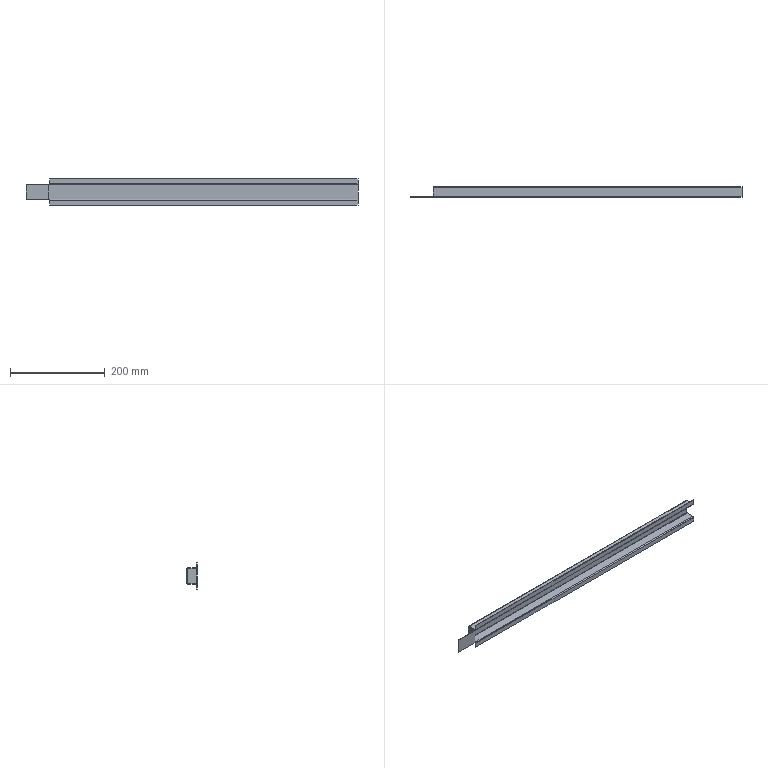Part | STEP file | 750078363 | 1 solid | 38 faces | box 699.5 x 21.5 x 55 mm | volume 93667 mm3 | plane 26 | cylinder 12 | commonest cylinder face diameters 1 x6 4 x6
STEP:
#1=CARTESIAN_POINT('',(-323.5,20.,15.));
#2=VERTEX_POINT('',#1);
#3=CARTESIAN_POINT('',(-323.5,20.,-15.));
#4=VERTEX_POINT('',#3);
#5=CARTESIAN_POINT('',(-323.5,20.,15.));
#6=DIRECTION('',(0.,0.,-1.));
#7=VECTOR('',#6,1000.);
#8=LINE('',#5,#7);
#9=EDGE_CURVE('',#2,#4,#8,.T.);
#10=ORIENTED_EDGE('',*,*,#9,.F.);
#11=CARTESIAN_POINT('',(325.5,20.,15.));
#12=VERTEX_POINT('',#11);
#13=CARTESIAN_POINT('',(325.5,20.,15.));
#14=DIRECTION('',(-1.,0.,0.));
#15=VECTOR('',#14,1000.);
#16=LINE('',#13,#15);
#17=EDGE_CURVE('',#12,#2,#16,.T.);
#18=ORIENTED_EDGE('',*,*,#17,.F.);
#19=CARTESIAN_POINT('',(325.5,20.,-15.));
#20=VERTEX_POINT('',#19);
#21=CARTESIAN_POINT('',(325.5,20.,15.));
#22=DIRECTION('',(0.,0.,1.));
#23=VECTOR('',#22,1000.);
#24=LINE('',#21,#23);
#25=EDGE_CURVE('',#20,#12,#24,.T.);
#26=ORIENTED_EDGE('',*,*,#25,.F.);
#27=CARTESIAN_POINT('',(325.5,20.,-15.));
#28=DIRECTION('',(1.,0.,0.));
#29=VECTOR('',#28,1000.);
#30=LINE('',#27,#29);
#31=EDGE_CURVE('',#4,#20,#30,.T.);
#32=ORIENTED_EDGE('',*,*,#31,.F.);
#33=EDGE_LOOP('',(#10,#18,#26,#32));
#34=FACE_OUTER_BOUND('',#33,.T.);
#35=CARTESIAN_POINT('',(325.5,20.,15.));
#36=DIRECTION('',(0.,-1.,0.));
#37=DIRECTION('',(1.,0.,0.));
#38=AXIS2_PLACEMENT_3D('',#35,#36,#37);
#39=PLANE('',#38);
#40=ADVANCED_FACE('',(#34),#39,.F.);
#41=CARTESIAN_POINT('',(325.5,18.,-17.));
#42=VERTEX_POINT('',#41);
#43=CARTESIAN_POINT('',(-323.998,18.,-17.));
#44=VERTEX_POINT('',#43);
#45=CARTESIAN_POINT('',(-323.5,18.,-17.));
#46=DIRECTION('',(-1.,0.,0.));
#47=VECTOR('',#46,1000.);
#48=LINE('',#45,#47);
#49=EDGE_CURVE('',#42,#44,#48,.T.);
#50=ORIENTED_EDGE('',*,*,#49,.T.);
#51=CARTESIAN_POINT('',(-323.998,19.936,-15.5));
#52=VERTEX_POINT('',#51);
#53=CARTESIAN_POINT('',(-323.998,18.,-15.));
#54=DIRECTION('',(1.,0.,0.));
#55=DIRECTION('',(0.,1.,0.));
#56=AXIS2_PLACEMENT_3D('',#53,#54,#55);
#57=CIRCLE('',#56,2.);
#58=EDGE_CURVE('',#44,#52,#57,.T.);
#59=ORIENTED_EDGE('',*,*,#58,.T.);
#60=CARTESIAN_POINT('',(-323.5,20.,-15.));
#61=CARTESIAN_POINT('',(-323.668,20.,-15.169));
#62=CARTESIAN_POINT('',(-323.835,19.979,-15.336));
#63=CARTESIAN_POINT('',(-323.998,19.936,-15.5));
#64=(BOUNDED_CURVE()B_SPLINE_CURVE(3,(#60,#61,#62,#63),.UNSPECIFIED.,.F.,.F.)B_SPLINE_CURVE_WITH_KNOTS((4,4),(1.571,1.823),.UNSPECIFIED.)CURVE()GEOMETRIC_REPRESENTATION_ITEM()RATIONAL_B_SPLINE_CURVE((1.,0.9947,0.9947,1.))REPRESENTATION_ITEM(''));
#65=EDGE_CURVE('',#4,#52,#64,.T.);
#66=ORIENTED_EDGE('',*,*,#65,.F.);
#67=ORIENTED_EDGE('',*,*,#31,.T.);
#68=CARTESIAN_POINT('',(325.5,18.,-15.));
#69=DIRECTION('',(-1.,0.,0.));
#70=DIRECTION('',(0.,1.,0.));
#71=AXIS2_PLACEMENT_3D('',#68,#69,#70);
#72=CIRCLE('',#71,2.);
#73=EDGE_CURVE('',#20,#42,#72,.T.);
#74=ORIENTED_EDGE('',*,*,#73,.T.);
#75=EDGE_LOOP('',(#50,#59,#66,#67,#74));
#76=FACE_OUTER_BOUND('',#75,.T.);
#77=CARTESIAN_POINT('',(-323.5,18.,-15.));
#78=DIRECTION('',(1.,0.,0.));
#79=DIRECTION('',(0.,1.,0.));
#80=AXIS2_PLACEMENT_3D('',#77,#78,#79);
#81=CYLINDRICAL_SURFACE('',#80,2.);
#82=ADVANCED_FACE('',(#76),#81,.T.);
#83=CARTESIAN_POINT('',(-325.5,18.,-15.498));
#84=VERTEX_POINT('',#83);
#85=CARTESIAN_POINT('',(-325.5,18.,15.498));
#86=VERTEX_POINT('',#85);
#87=CARTESIAN_POINT('',(-325.5,18.,15.));
#88=DIRECTION('',(0.,0.,1.));
#89=VECTOR('',#88,1000.);
#90=LINE('',#87,#89);
#91=EDGE_CURVE('',#84,#86,#90,.T.);
#92=ORIENTED_EDGE('',*,*,#91,.T.);
#93=CARTESIAN_POINT('',(-324.,19.936,15.498));
#94=VERTEX_POINT('',#93);
#95=CARTESIAN_POINT('',(-323.5,18.,15.498));
#96=DIRECTION('',(0.,0.,-1.));
#97=DIRECTION('',(-1.,0.,0.));
#98=AXIS2_PLACEMENT_3D('',#95,#96,#97);
#99=CIRCLE('',#98,2.);
#100=EDGE_CURVE('',#86,#94,#99,.T.);
#101=ORIENTED_EDGE('',*,*,#100,.T.);
#102=CARTESIAN_POINT('',(-323.5,20.,15.));
#103=CARTESIAN_POINT('',(-323.669,20.,15.168));
#104=CARTESIAN_POINT('',(-323.836,19.979,15.335));
#105=CARTESIAN_POINT('',(-324.,19.936,15.498));
#106=(BOUNDED_CURVE()B_SPLINE_CURVE(3,(#102,#103,#104,#105),.UNSPECIFIED.,.F.,.F.)B_SPLINE_CURVE_WITH_KNOTS((4,4),(1.571,1.823),.UNSPECIFIED.)CURVE()GEOMETRIC_REPRESENTATION_ITEM()RATIONAL_B_SPLINE_CURVE((1.,0.9947,0.9947,1.))REPRESENTATION_ITEM(''));
#107=EDGE_CURVE('',#2,#94,#106,.T.);
#108=ORIENTED_EDGE('',*,*,#107,.F.);
#109=ORIENTED_EDGE('',*,*,#9,.T.);
#110=CARTESIAN_POINT('',(-324.,19.936,-15.498));
#111=VERTEX_POINT('',#110);
#112=CARTESIAN_POINT('',(-323.5,20.,-15.));
#113=CARTESIAN_POINT('',(-323.669,20.,-15.168));
#114=CARTESIAN_POINT('',(-323.836,19.979,-15.335));
#115=CARTESIAN_POINT('',(-324.,19.936,-15.498));
#116=(BOUNDED_CURVE()B_SPLINE_CURVE(3,(#112,#113,#114,#115),.UNSPECIFIED.,.F.,.F.)B_SPLINE_CURVE_WITH_KNOTS((4,4),(4.712,4.965),.UNSPECIFIED.)CURVE()GEOMETRIC_REPRESENTATION_ITEM()RATIONAL_B_SPLINE_CURVE((1.,0.9947,0.9947,1.))REPRESENTATION_ITEM(''));
#117=EDGE_CURVE('',#4,#111,#116,.T.);
#118=ORIENTED_EDGE('',*,*,#117,.T.);
#119=CARTESIAN_POINT('',(-323.5,18.,-15.498));
#120=DIRECTION('',(0.,0.,1.));
#121=DIRECTION('',(-1.,0.,0.));
#122=AXIS2_PLACEMENT_3D('',#119,#120,#121);
#123=CIRCLE('',#122,2.);
#124=EDGE_CURVE('',#111,#84,#123,.T.);
#125=ORIENTED_EDGE('',*,*,#124,.T.);
#126=EDGE_LOOP('',(#92,#101,#108,#109,#118,#125));
#127=FACE_OUTER_BOUND('',#126,.T.);
#128=CARTESIAN_POINT('',(-323.5,18.,15.));
#129=DIRECTION('',(0.,0.,-1.));
#130=DIRECTION('',(-1.,0.,0.));
#131=AXIS2_PLACEMENT_3D('',#128,#129,#130);
#132=CYLINDRICAL_SURFACE('',#131,2.);
#133=ADVANCED_FACE('',(#127),#132,.T.);
#134=CARTESIAN_POINT('',(-323.998,18.,17.));
#135=VERTEX_POINT('',#134);
#136=CARTESIAN_POINT('',(325.5,18.,17.));
#137=VERTEX_POINT('',#136);
#138=CARTESIAN_POINT('',(325.5,18.,17.));
#139=DIRECTION('',(1.,0.,0.));
#140=VECTOR('',#139,1000.);
#141=LINE('',#138,#140);
#142=EDGE_CURVE('',#135,#137,#141,.T.);
#143=ORIENTED_EDGE('',*,*,#142,.T.);
#144=CARTESIAN_POINT('',(325.5,18.,15.));
#145=DIRECTION('',(-1.,0.,0.));
#146=DIRECTION('',(0.,-1.,0.));
#147=AXIS2_PLACEMENT_3D('',#144,#145,#146);
#148=CIRCLE('',#147,2.);
#149=EDGE_CURVE('',#137,#12,#148,.T.);
#150=ORIENTED_EDGE('',*,*,#149,.T.);
#151=ORIENTED_EDGE('',*,*,#17,.T.);
#152=CARTESIAN_POINT('',(-323.998,19.936,15.5));
#153=VERTEX_POINT('',#152);
#154=CARTESIAN_POINT('',(-323.5,20.,15.));
#155=CARTESIAN_POINT('',(-323.668,20.,15.169));
#156=CARTESIAN_POINT('',(-323.835,19.979,15.336));
#157=CARTESIAN_POINT('',(-323.998,19.936,15.5));
#158=(BOUNDED_CURVE()B_SPLINE_CURVE(3,(#154,#155,#156,#157),.UNSPECIFIED.,.F.,.F.)B_SPLINE_CURVE_WITH_KNOTS((4,4),(4.712,4.965),.UNSPECIFIED.)CURVE()GEOMETRIC_REPRESENTATION_ITEM()RATIONAL_B_SPLINE_CURVE((1.,0.9947,0.9947,1.))REPRESENTATION_ITEM(''));
#159=EDGE_CURVE('',#2,#153,#158,.T.);
#160=ORIENTED_EDGE('',*,*,#159,.T.);
#161=CARTESIAN_POINT('',(-323.998,18.,15.));
#162=DIRECTION('',(1.,0.,0.));
#163=DIRECTION('',(0.,-1.,0.));
#164=AXIS2_PLACEMENT_3D('',#161,#162,#163);
#165=CIRCLE('',#164,2.);
#166=EDGE_CURVE('',#153,#135,#165,.T.);
#167=ORIENTED_EDGE('',*,*,#166,.T.);
#168=EDGE_LOOP('',(#143,#150,#151,#160,#167));
#169=FACE_OUTER_BOUND('',#168,.T.);
#170=CARTESIAN_POINT('',(325.5,18.,15.));
#171=DIRECTION('',(-1.,0.,0.));
#172=DIRECTION('',(0.,-1.,0.));
#173=AXIS2_PLACEMENT_3D('',#170,#171,#172);
#174=CYLINDRICAL_SURFACE('',#173,2.);
#175=ADVANCED_FACE('',(#169),#174,.T.);
#176=ORIENTED_EDGE('',*,*,#25,.T.);
#177=ORIENTED_EDGE('',*,*,#149,.F.);
#178=CARTESIAN_POINT('',(325.5,0.5,17.));
#179=VERTEX_POINT('',#178);
#180=CARTESIAN_POINT('',(325.5,20.,17.));
#181=DIRECTION('',(0.,1.,0.));
#182=VECTOR('',#181,1000.);
#183=LINE('',#180,#182);
#184=EDGE_CURVE('',#179,#137,#183,.T.);
#185=ORIENTED_EDGE('',*,*,#184,.F.);
#186=CARTESIAN_POINT('',(325.5,0.,17.5));
#187=VERTEX_POINT('',#186);
#188=CARTESIAN_POINT('',(325.5,0.5,17.5));
#189=DIRECTION('',(-1.,0.,0.));
#190=DIRECTION('',(0.,1.,0.));
#191=AXIS2_PLACEMENT_3D('',#188,#189,#190);
#192=CIRCLE('',#191,0.5);
#193=EDGE_CURVE('',#179,#187,#192,.T.);
#194=ORIENTED_EDGE('',*,*,#193,.T.);
#195=CARTESIAN_POINT('',(325.5,0.,27.5));
#196=VERTEX_POINT('',#195);
#197=CARTESIAN_POINT('',(325.5,0.,15.));
#198=DIRECTION('',(0.,0.,-1.));
#199=VECTOR('',#198,1000.);
#200=LINE('',#197,#199);
#201=EDGE_CURVE('',#196,#187,#200,.T.);
#202=ORIENTED_EDGE('',*,*,#201,.F.);
#203=CARTESIAN_POINT('',(325.5,-1.5,27.5));
#204=VERTEX_POINT('',#203);
#205=CARTESIAN_POINT('',(325.5,0.,27.5));
#206=DIRECTION('',(0.,1.,0.));
#207=VECTOR('',#206,1000.);
#208=LINE('',#205,#207);
#209=EDGE_CURVE('',#204,#196,#208,.T.);
#210=ORIENTED_EDGE('',*,*,#209,.F.);
#211=CARTESIAN_POINT('',(325.5,-1.5,17.5));
#212=VERTEX_POINT('',#211);
#213=CARTESIAN_POINT('',(325.5,-1.5,15.));
#214=DIRECTION('',(0.,0.,1.));
#215=VECTOR('',#214,1000.);
#216=LINE('',#213,#215);
#217=EDGE_CURVE('',#212,#204,#216,.T.);
#218=ORIENTED_EDGE('',*,*,#217,.F.);
#219=CARTESIAN_POINT('',(325.5,0.5,15.5));
#220=VERTEX_POINT('',#219);
#221=CARTESIAN_POINT('',(325.5,0.5,17.5));
#222=DIRECTION('',(-1.,0.,0.));
#223=DIRECTION('',(0.,1.,0.));
#224=AXIS2_PLACEMENT_3D('',#221,#222,#223);
#225=CIRCLE('',#224,2.);
#226=EDGE_CURVE('',#220,#212,#225,.T.);
#227=ORIENTED_EDGE('',*,*,#226,.F.);
#228=CARTESIAN_POINT('',(325.5,18.,15.5));
#229=VERTEX_POINT('',#228);
#230=CARTESIAN_POINT('',(325.5,20.,15.5));
#231=DIRECTION('',(0.,-1.,0.));
#232=VECTOR('',#231,1000.);
#233=LINE('',#230,#232);
#234=EDGE_CURVE('',#229,#220,#233,.T.);
#235=ORIENTED_EDGE('',*,*,#234,.F.);
#236=CARTESIAN_POINT('',(325.5,18.5,15.));
#237=VERTEX_POINT('',#236);
#238=CARTESIAN_POINT('',(325.5,18.,15.));
#239=DIRECTION('',(-1.,0.,0.));
#240=DIRECTION('',(0.,-1.,0.));
#241=AXIS2_PLACEMENT_3D('',#238,#239,#240);
#242=CIRCLE('',#241,0.5);
#243=EDGE_CURVE('',#229,#237,#242,.T.);
#244=ORIENTED_EDGE('',*,*,#243,.T.);
#245=CARTESIAN_POINT('',(325.5,18.5,-15.));
#246=VERTEX_POINT('',#245);
#247=CARTESIAN_POINT('',(325.5,18.5,15.));
#248=DIRECTION('',(0.,0.,1.));
#249=VECTOR('',#248,1000.);
#250=LINE('',#247,#249);
#251=EDGE_CURVE('',#246,#237,#250,.T.);
#252=ORIENTED_EDGE('',*,*,#251,.F.);
#253=CARTESIAN_POINT('',(325.5,18.,-15.5));
#254=VERTEX_POINT('',#253);
#255=CARTESIAN_POINT('',(325.5,18.,-15.));
#256=DIRECTION('',(-1.,0.,0.));
#257=DIRECTION('',(0.,1.,0.));
#258=AXIS2_PLACEMENT_3D('',#255,#256,#257);
#259=CIRCLE('',#258,0.5);
#260=EDGE_CURVE('',#246,#254,#259,.T.);
#261=ORIENTED_EDGE('',*,*,#260,.T.);
#262=CARTESIAN_POINT('',(325.5,0.5,-15.5));
#263=VERTEX_POINT('',#262);
#264=CARTESIAN_POINT('',(325.5,20.,-15.5));
#265=DIRECTION('',(0.,1.,0.));
#266=VECTOR('',#265,1000.);
#267=LINE('',#264,#266);
#268=EDGE_CURVE('',#263,#254,#267,.T.);
#269=ORIENTED_EDGE('',*,*,#268,.F.);
#270=CARTESIAN_POINT('',(325.5,-1.5,-17.5));
#271=VERTEX_POINT('',#270);
#272=CARTESIAN_POINT('',(325.5,0.5,-17.5));
#273=DIRECTION('',(-1.,0.,0.));
#274=DIRECTION('',(0.,-1.,0.));
#275=AXIS2_PLACEMENT_3D('',#272,#273,#274);
#276=CIRCLE('',#275,2.);
#277=EDGE_CURVE('',#271,#263,#276,.T.);
#278=ORIENTED_EDGE('',*,*,#277,.F.);
#279=CARTESIAN_POINT('',(325.5,-1.5,-27.5));
#280=VERTEX_POINT('',#279);
#281=CARTESIAN_POINT('',(325.5,-1.5,15.));
#282=DIRECTION('',(0.,0.,1.));
#283=VECTOR('',#282,1000.);
#284=LINE('',#281,#283);
#285=EDGE_CURVE('',#280,#271,#284,.T.);
#286=ORIENTED_EDGE('',*,*,#285,.F.);
#287=CARTESIAN_POINT('',(325.5,0.,-27.5));
#288=VERTEX_POINT('',#287);
#289=CARTESIAN_POINT('',(325.5,0.,-27.5));
#290=DIRECTION('',(0.,-1.,0.));
#291=VECTOR('',#290,1000.);
#292=LINE('',#289,#291);
#293=EDGE_CURVE('',#288,#280,#292,.T.);
#294=ORIENTED_EDGE('',*,*,#293,.F.);
#295=CARTESIAN_POINT('',(325.5,0.,-17.5));
#296=VERTEX_POINT('',#295);
#297=CARTESIAN_POINT('',(325.5,0.,15.));
#298=DIRECTION('',(0.,0.,-1.));
#299=VECTOR('',#298,1000.);
#300=LINE('',#297,#299);
#301=EDGE_CURVE('',#296,#288,#300,.T.);
#302=ORIENTED_EDGE('',*,*,#301,.F.);
#303=CARTESIAN_POINT('',(325.5,0.5,-17.));
#304=VERTEX_POINT('',#303);
#305=CARTESIAN_POINT('',(325.5,0.5,-17.5));
#306=DIRECTION('',(1.,0.,0.));
#307=DIRECTION('',(0.,-1.,0.));
#308=AXIS2_PLACEMENT_3D('',#305,#306,#307);
#309=CIRCLE('',#308,0.5);
#310=EDGE_CURVE('',#304,#296,#309,.T.);
#311=ORIENTED_EDGE('',*,*,#310,.F.);
#312=CARTESIAN_POINT('',(325.5,18.,-17.));
#313=DIRECTION('',(0.,1.,0.));
#314=VECTOR('',#313,1000.);
#315=LINE('',#312,#314);
#316=EDGE_CURVE('',#304,#42,#315,.T.);
#317=ORIENTED_EDGE('',*,*,#316,.T.);
#318=ORIENTED_EDGE('',*,*,#73,.F.);
#319=EDGE_LOOP('',(#176,#177,#185,#194,#202,#210,#218,#227,#235,#244,#252,#261,#269,#278,#286,#294,#302,#311,#317,#318));
#320=FACE_OUTER_BOUND('',#319,.T.);
#321=CARTESIAN_POINT('',(325.5,20.,15.));
#322=DIRECTION('',(-1.,0.,0.));
#323=DIRECTION('',(0.,-1.,0.));
#324=AXIS2_PLACEMENT_3D('',#321,#322,#323);
#325=PLANE('',#324);
#326=ADVANCED_FACE('',(#320),#325,.F.);
#327=CARTESIAN_POINT('',(-323.998,-1.5,-27.5));
#328=VERTEX_POINT('',#327);
#329=CARTESIAN_POINT('',(-323.998,-1.5,-17.5));
#330=VERTEX_POINT('',#329);
#331=CARTESIAN_POINT('',(-323.998,-1.5,-15.5));
#332=DIRECTION('',(0.,0.,1.));
#333=VECTOR('',#332,1000.);
#334=LINE('',#331,#333);
#335=EDGE_CURVE('',#328,#330,#334,.T.);
#336=ORIENTED_EDGE('',*,*,#335,.T.);
#337=CARTESIAN_POINT('',(-323.998,0.5,-15.5));
#338=VERTEX_POINT('',#337);
#339=CARTESIAN_POINT('',(-323.998,0.5,-17.5));
#340=DIRECTION('',(-1.,0.,0.));
#341=DIRECTION('',(0.,-1.,0.));
#342=AXIS2_PLACEMENT_3D('',#339,#340,#341);
#343=CIRCLE('',#342,2.);
#344=EDGE_CURVE('',#330,#338,#343,.T.);
#345=ORIENTED_EDGE('',*,*,#344,.T.);
#346=CARTESIAN_POINT('',(-323.998,18.,-15.5));
#347=VERTEX_POINT('',#346);
#348=CARTESIAN_POINT('',(-323.998,18.,-15.5));
#349=DIRECTION('',(0.,1.,0.));
#350=VECTOR('',#349,1000.);
#351=LINE('',#348,#350);
#352=EDGE_CURVE('',#338,#347,#351,.T.);
#353=ORIENTED_EDGE('',*,*,#352,.T.);
#354=CARTESIAN_POINT('',(-323.998,18.,-15.5));
#355=DIRECTION('',(0.,1.,0.));
#356=VECTOR('',#355,1000.);
#357=LINE('',#354,#356);
#358=EDGE_CURVE('',#347,#52,#357,.T.);
#359=ORIENTED_EDGE('',*,*,#358,.T.);
#360=ORIENTED_EDGE('',*,*,#58,.F.);
#361=CARTESIAN_POINT('',(-323.998,0.5,-17.));
#362=VERTEX_POINT('',#361);
#363=CARTESIAN_POINT('',(-323.998,18.,-17.));
#364=DIRECTION('',(0.,-1.,0.));
#365=VECTOR('',#364,1000.);
#366=LINE('',#363,#365);
#367=EDGE_CURVE('',#44,#362,#366,.T.);
#368=ORIENTED_EDGE('',*,*,#367,.T.);
#369=CARTESIAN_POINT('',(-323.998,0.,-17.5));
#370=VERTEX_POINT('',#369);
#371=CARTESIAN_POINT('',(-323.998,0.5,-17.5));
#372=DIRECTION('',(1.,0.,0.));
#373=DIRECTION('',(0.,-1.,0.));
#374=AXIS2_PLACEMENT_3D('',#371,#372,#373);
#375=CIRCLE('',#374,0.5);
#376=EDGE_CURVE('',#362,#370,#375,.T.);
#377=ORIENTED_EDGE('',*,*,#376,.T.);
#378=CARTESIAN_POINT('',(-323.998,0.,-27.5));
#379=VERTEX_POINT('',#378);
#380=CARTESIAN_POINT('',(-323.998,0.,-15.5));
#381=DIRECTION('',(0.,0.,-1.));
#382=VECTOR('',#381,1000.);
#383=LINE('',#380,#382);
#384=EDGE_CURVE('',#370,#379,#383,.T.);
#385=ORIENTED_EDGE('',*,*,#384,.T.);
#386=CARTESIAN_POINT('',(-323.998,0.,-27.5));
#387=DIRECTION('',(0.,1.,0.));
#388=VECTOR('',#387,1000.);
#389=LINE('',#386,#388);
#390=EDGE_CURVE('',#328,#379,#389,.T.);
#391=ORIENTED_EDGE('',*,*,#390,.F.);
#392=EDGE_LOOP('',(#336,#345,#353,#359,#360,#368,#377,#385,#391));
#393=FACE_OUTER_BOUND('',#392,.T.);
#394=CARTESIAN_POINT('',(-323.998,18.,-15.5));
#395=DIRECTION('',(-1.,0.,0.));
#396=DIRECTION('',(0.,0.,1.));
#397=AXIS2_PLACEMENT_3D('',#394,#395,#396);
#398=PLANE('',#397);
#399=ADVANCED_FACE('',(#393),#398,.T.);
#400=CARTESIAN_POINT('',(-323.5,0.5,-17.));
#401=DIRECTION('',(1.,0.,0.));
#402=VECTOR('',#401,1000.);
#403=LINE('',#400,#402);
#404=EDGE_CURVE('',#362,#304,#403,.T.);
#405=ORIENTED_EDGE('',*,*,#404,.F.);
#406=ORIENTED_EDGE('',*,*,#367,.F.);
#407=ORIENTED_EDGE('',*,*,#49,.F.);
#408=ORIENTED_EDGE('',*,*,#316,.F.);
#409=EDGE_LOOP('',(#405,#406,#407,#408));
#410=FACE_OUTER_BOUND('',#409,.T.);
#411=CARTESIAN_POINT('',(-323.5,18.,-17.));
#412=DIRECTION('',(0.,0.,1.));
#413=DIRECTION('',(0.,-1.,0.));
#414=AXIS2_PLACEMENT_3D('',#411,#412,#413);
#415=PLANE('',#414);
#416=ADVANCED_FACE('',(#410),#415,.F.);
#417=CARTESIAN_POINT('',(-374.,-1.5,15.498));
#418=VERTEX_POINT('',#417);
#419=CARTESIAN_POINT('',(-326.,-1.5,15.498));
#420=VERTEX_POINT('',#419);
#421=CARTESIAN_POINT('',(-325.5,-1.5,15.498));
#422=DIRECTION('',(1.,0.,0.));
#423=VECTOR('',#422,1000.);
#424=LINE('',#421,#423);
#425=EDGE_CURVE('',#418,#420,#424,.T.);
#426=ORIENTED_EDGE('',*,*,#425,.T.);
#427=CARTESIAN_POINT('',(-324.,0.5,15.498));
#428=VERTEX_POINT('',#427);
#429=CARTESIAN_POINT('',(-326.,0.5,15.498));
#430=DIRECTION('',(0.,0.,1.));
#431=DIRECTION('',(-1.,0.,0.));
#432=AXIS2_PLACEMENT_3D('',#429,#430,#431);
#433=CIRCLE('',#432,2.);
#434=EDGE_CURVE('',#420,#428,#433,.T.);
#435=ORIENTED_EDGE('',*,*,#434,.T.);
#436=CARTESIAN_POINT('',(-324.,18.,15.498));
#437=VERTEX_POINT('',#436);
#438=CARTESIAN_POINT('',(-324.,0.,15.498));
#439=DIRECTION('',(0.,1.,0.));
#440=VECTOR('',#439,1000.);
#441=LINE('',#438,#440);
#442=EDGE_CURVE('',#428,#437,#441,.T.);
#443=ORIENTED_EDGE('',*,*,#442,.T.);
#444=CARTESIAN_POINT('',(-324.,0.,15.498));
#445=DIRECTION('',(0.,1.,0.));
#446=VECTOR('',#445,1000.);
#447=LINE('',#444,#446);
#448=EDGE_CURVE('',#437,#94,#447,.T.);
#449=ORIENTED_EDGE('',*,*,#448,.T.);
#450=ORIENTED_EDGE('',*,*,#100,.F.);
#451=CARTESIAN_POINT('',(-325.5,0.5,15.498));
#452=VERTEX_POINT('',#451);
#453=CARTESIAN_POINT('',(-325.5,0.,15.498));
#454=DIRECTION('',(0.,-1.,0.));
#455=VECTOR('',#454,1000.);
#456=LINE('',#453,#455);
#457=EDGE_CURVE('',#86,#452,#456,.T.);
#458=ORIENTED_EDGE('',*,*,#457,.T.);
#459=CARTESIAN_POINT('',(-326.,0.,15.498));
#460=VERTEX_POINT('',#459);
#461=CARTESIAN_POINT('',(-326.,0.5,15.498));
#462=DIRECTION('',(0.,0.,-1.));
#463=DIRECTION('',(-1.,0.,0.));
#464=AXIS2_PLACEMENT_3D('',#461,#462,#463);
#465=CIRCLE('',#464,0.5);
#466=EDGE_CURVE('',#452,#460,#465,.T.);
#467=ORIENTED_EDGE('',*,*,#466,.T.);
#468=CARTESIAN_POINT('',(-374.,0.,15.498));
#469=VERTEX_POINT('',#468);
#470=CARTESIAN_POINT('',(-325.5,0.,15.498));
#471=DIRECTION('',(-1.,0.,0.));
#472=VECTOR('',#471,1000.);
#473=LINE('',#470,#472);
#474=EDGE_CURVE('',#460,#469,#473,.T.);
#475=ORIENTED_EDGE('',*,*,#474,.T.);
#476=CARTESIAN_POINT('',(-374.,0.,15.498));
#477=DIRECTION('',(0.,1.,0.));
#478=VECTOR('',#477,1000.);
#479=LINE('',#476,#478);
#480=EDGE_CURVE('',#418,#469,#479,.T.);
#481=ORIENTED_EDGE('',*,*,#480,.F.);
#482=EDGE_LOOP('',(#426,#435,#443,#449,#450,#458,#467,#475,#481));
#483=FACE_OUTER_BOUND('',#482,.T.);
#484=CARTESIAN_POINT('',(-325.5,0.,15.498));
#485=DIRECTION('',(0.,0.,1.));
#486=DIRECTION('',(1.,0.,0.));
#487=AXIS2_PLACEMENT_3D('',#484,#485,#486);
#488=PLANE('',#487);
#489=ADVANCED_FACE('',(#483),#488,.T.);
#490=CARTESIAN_POINT('',(-325.5,0.5,-15.498));
#491=VERTEX_POINT('',#490);
#492=CARTESIAN_POINT('',(-325.5,0.5,15.));
#493=DIRECTION('',(0.,0.,-1.));
#494=VECTOR('',#493,1000.);
#495=LINE('',#492,#494);
#496=EDGE_CURVE('',#452,#491,#495,.T.);
#497=ORIENTED_EDGE('',*,*,#496,.F.);
#498=ORIENTED_EDGE('',*,*,#457,.F.);
#499=ORIENTED_EDGE('',*,*,#91,.F.);
#500=CARTESIAN_POINT('',(-325.5,20.,-15.498));
#501=DIRECTION('',(0.,1.,0.));
#502=VECTOR('',#501,1000.);
#503=LINE('',#500,#502);
#504=EDGE_CURVE('',#491,#84,#503,.T.);
#505=ORIENTED_EDGE('',*,*,#504,.F.);
#506=EDGE_LOOP('',(#497,#498,#499,#505));
#507=FACE_OUTER_BOUND('',#506,.T.);
#508=CARTESIAN_POINT('',(-325.5,20.,15.));
#509=DIRECTION('',(1.,0.,0.));
#510=DIRECTION('',(0.,0.,-1.));
#511=AXIS2_PLACEMENT_3D('',#508,#509,#510);
#512=PLANE('',#511);
#513=ADVANCED_FACE('',(#507),#512,.F.);
#514=ORIENTED_EDGE('',*,*,#124,.F.);
#515=CARTESIAN_POINT('',(-324.,18.,-15.498));
#516=VERTEX_POINT('',#515);
#517=CARTESIAN_POINT('',(-324.,20.,-15.498));
#518=DIRECTION('',(0.,1.,0.));
#519=VECTOR('',#518,1000.);
#520=LINE('',#517,#519);
#521=EDGE_CURVE('',#516,#111,#520,.T.);
#522=ORIENTED_EDGE('',*,*,#521,.F.);
#523=CARTESIAN_POINT('',(-324.,0.5,-15.498));
#524=VERTEX_POINT('',#523);
#525=CARTESIAN_POINT('',(-324.,20.,-15.498));
#526=DIRECTION('',(0.,1.,0.));
#527=VECTOR('',#526,1000.);
#528=LINE('',#525,#527);
#529=EDGE_CURVE('',#524,#516,#528,.T.);
#530=ORIENTED_EDGE('',*,*,#529,.F.);
#531=CARTESIAN_POINT('',(-326.,-1.5,-15.498));
#532=VERTEX_POINT('',#531);
#533=CARTESIAN_POINT('',(-326.,0.5,-15.498));
#534=DIRECTION('',(0.,0.,1.));
#535=DIRECTION('',(-1.,0.,0.));
#536=AXIS2_PLACEMENT_3D('',#533,#534,#535);
#537=CIRCLE('',#536,2.);
#538=EDGE_CURVE('',#532,#524,#537,.T.);
#539=ORIENTED_EDGE('',*,*,#538,.F.);
#540=CARTESIAN_POINT('',(-374.,-1.5,-15.498));
#541=VERTEX_POINT('',#540);
#542=CARTESIAN_POINT('',(325.5,-1.5,-15.498));
#543=DIRECTION('',(1.,0.,0.));
#544=VECTOR('',#543,1000.);
#545=LINE('',#542,#544);
#546=EDGE_CURVE('',#541,#532,#545,.T.);
#547=ORIENTED_EDGE('',*,*,#546,.F.);
#548=CARTESIAN_POINT('',(-374.,0.,-15.498));
#549=VERTEX_POINT('',#548);
#550=CARTESIAN_POINT('',(-374.,0.,-15.498));
#551=DIRECTION('',(0.,-1.,0.));
#552=VECTOR('',#551,1000.);
#553=LINE('',#550,#552);
#554=EDGE_CURVE('',#549,#541,#553,.T.);
#555=ORIENTED_EDGE('',*,*,#554,.F.);
#556=CARTESIAN_POINT('',(-326.,0.,-15.498));
#557=VERTEX_POINT('',#556);
#558=CARTESIAN_POINT('',(325.5,0.,-15.498));
#559=DIRECTION('',(-1.,0.,0.));
#560=VECTOR('',#559,1000.);
#561=LINE('',#558,#560);
#562=EDGE_CURVE('',#557,#549,#561,.T.);
#563=ORIENTED_EDGE('',*,*,#562,.F.);
#564=CARTESIAN_POINT('',(-326.,0.5,-15.498));
#565=DIRECTION('',(0.,0.,-1.));
#566=DIRECTION('',(-1.,0.,0.));
#567=AXIS2_PLACEMENT_3D('',#564,#565,#566);
#568=CIRCLE('',#567,0.5);
#569=EDGE_CURVE('',#491,#557,#568,.T.);
#570=ORIENTED_EDGE('',*,*,#569,.F.);
#571=ORIENTED_EDGE('',*,*,#504,.T.);
#572=EDGE_LOOP('',(#514,#522,#530,#539,#547,#555,#563,#570,#571));
#573=FACE_OUTER_BOUND('',#572,.T.);
#574=CARTESIAN_POINT('',(325.5,20.,-15.498));
#575=DIRECTION('',(0.,0.,1.));
#576=DIRECTION('',(1.,0.,0.));
#577=AXIS2_PLACEMENT_3D('',#574,#575,#576);
#578=PLANE('',#577);
#579=ADVANCED_FACE('',(#573),#578,.F.);
#580=CARTESIAN_POINT('',(-323.998,0.5,17.));
#581=VERTEX_POINT('',#580);
#582=CARTESIAN_POINT('',(325.5,0.5,17.));
#583=DIRECTION('',(-1.,0.,0.));
#584=VECTOR('',#583,1000.);
#585=LINE('',#582,#584);
#586=EDGE_CURVE('',#179,#581,#585,.T.);
#587=ORIENTED_EDGE('',*,*,#586,.F.);
#588=ORIENTED_EDGE('',*,*,#184,.T.);
#589=ORIENTED_EDGE('',*,*,#142,.F.);
#590=CARTESIAN_POINT('',(-323.998,18.,17.));
#591=DIRECTION('',(0.,1.,0.));
#592=VECTOR('',#591,1000.);
#593=LINE('',#590,#592);
#594=EDGE_CURVE('',#581,#135,#593,.T.);
#595=ORIENTED_EDGE('',*,*,#594,.F.);
#596=EDGE_LOOP('',(#587,#588,#589,#595));
#597=FACE_OUTER_BOUND('',#596,.T.);
#598=CARTESIAN_POINT('',(325.5,18.,17.));
#599=DIRECTION('',(0.,0.,-1.));
#600=DIRECTION('',(0.,1.,0.));
#601=AXIS2_PLACEMENT_3D('',#598,#599,#600);
#602=PLANE('',#601);
#603=ADVANCED_FACE('',(#597),#602,.F.);
#604=CARTESIAN_POINT('',(-323.998,0.,27.5));
#605=VERTEX_POINT('',#604);
#606=CARTESIAN_POINT('',(-323.998,0.,17.5));
#607=VERTEX_POINT('',#606);
#608=CARTESIAN_POINT('',(-323.998,0.,15.));
#609=DIRECTION('',(0.,0.,-1.));
#610=VECTOR('',#609,1000.);
#611=LINE('',#608,#610);
#612=EDGE_CURVE('',#605,#607,#611,.T.);
#613=ORIENTED_EDGE('',*,*,#612,.T.);
#614=CARTESIAN_POINT('',(-323.998,0.5,17.5));
#615=DIRECTION('',(1.,0.,0.));
#616=DIRECTION('',(0.,1.,0.));
#617=AXIS2_PLACEMENT_3D('',#614,#615,#616);
#618=CIRCLE('',#617,0.5);
#619=EDGE_CURVE('',#607,#581,#618,.T.);
#620=ORIENTED_EDGE('',*,*,#619,.T.);
#621=ORIENTED_EDGE('',*,*,#594,.T.);
#622=ORIENTED_EDGE('',*,*,#166,.F.);
#623=CARTESIAN_POINT('',(-323.998,18.,15.5));
#624=VERTEX_POINT('',#623);
#625=CARTESIAN_POINT('',(-323.998,18.,15.5));
#626=DIRECTION('',(0.,-1.,0.));
#627=VECTOR('',#626,1000.);
#628=LINE('',#625,#627);
#629=EDGE_CURVE('',#153,#624,#628,.T.);
#630=ORIENTED_EDGE('',*,*,#629,.T.);
#631=CARTESIAN_POINT('',(-323.998,0.5,15.5));
#632=VERTEX_POINT('',#631);
#633=CARTESIAN_POINT('',(-323.998,18.,15.5));
#634=DIRECTION('',(0.,-1.,0.));
#635=VECTOR('',#634,1000.);
#636=LINE('',#633,#635);
#637=EDGE_CURVE('',#624,#632,#636,.T.);
#638=ORIENTED_EDGE('',*,*,#637,.T.);
#639=CARTESIAN_POINT('',(-323.998,-1.5,17.5));
#640=VERTEX_POINT('',#639);
#641=CARTESIAN_POINT('',(-323.998,0.5,17.5));
#642=DIRECTION('',(-1.,0.,0.));
#643=DIRECTION('',(0.,1.,0.));
#644=AXIS2_PLACEMENT_3D('',#641,#642,#643);
#645=CIRCLE('',#644,2.);
#646=EDGE_CURVE('',#632,#640,#645,.T.);
#647=ORIENTED_EDGE('',*,*,#646,.T.);
#648=CARTESIAN_POINT('',(-323.998,-1.5,27.5));
#649=VERTEX_POINT('',#648);
#650=CARTESIAN_POINT('',(-323.998,-1.5,15.));
#651=DIRECTION('',(0.,0.,1.));
#652=VECTOR('',#651,1000.);
#653=LINE('',#650,#652);
#654=EDGE_CURVE('',#640,#649,#653,.T.);
#655=ORIENTED_EDGE('',*,*,#654,.T.);
#656=CARTESIAN_POINT('',(-323.998,0.,27.5));
#657=DIRECTION('',(0.,-1.,0.));
#658=VECTOR('',#657,1000.);
#659=LINE('',#656,#658);
#660=EDGE_CURVE('',#605,#649,#659,.T.);
#661=ORIENTED_EDGE('',*,*,#660,.F.);
#662=EDGE_LOOP('',(#613,#620,#621,#622,#630,#638,#647,#655,#661));
#663=FACE_OUTER_BOUND('',#662,.T.);
#664=CARTESIAN_POINT('',(-323.998,18.,15.));
#665=DIRECTION('',(-1.,0.,0.));
#666=DIRECTION('',(0.,-1.,0.));
#667=AXIS2_PLACEMENT_3D('',#664,#665,#666);
#668=PLANE('',#667);
#669=ADVANCED_FACE('',(#663),#668,.T.);
#670=CARTESIAN_POINT('',(-323.5,18.5,15.));
#671=VERTEX_POINT('',#670);
#672=CARTESIAN_POINT('',(325.5,18.5,15.));
#673=DIRECTION('',(-1.,0.,0.));
#674=VECTOR('',#673,1000.);
#675=LINE('',#672,#674);
#676=EDGE_CURVE('',#237,#671,#675,.T.);
#677=ORIENTED_EDGE('',*,*,#676,.T.);
#678=CARTESIAN_POINT('',(-323.5,18.5,-15.));
#679=VERTEX_POINT('',#678);
#680=CARTESIAN_POINT('',(-323.5,18.5,15.));
#681=DIRECTION('',(0.,0.,-1.));
#682=VECTOR('',#681,1000.);
#683=LINE('',#680,#682);
#684=EDGE_CURVE('',#671,#679,#683,.T.);
#685=ORIENTED_EDGE('',*,*,#684,.T.);
#686=CARTESIAN_POINT('',(325.5,18.5,-15.));
#687=DIRECTION('',(1.,0.,0.));
#688=VECTOR('',#687,1000.);
#689=LINE('',#686,#688);
#690=EDGE_CURVE('',#679,#246,#689,.T.);
#691=ORIENTED_EDGE('',*,*,#690,.T.);
#692=ORIENTED_EDGE('',*,*,#251,.T.);
#693=EDGE_LOOP('',(#677,#685,#691,#692));
#694=FACE_OUTER_BOUND('',#693,.T.);
#695=CARTESIAN_POINT('',(325.5,18.5,15.));
#696=DIRECTION('',(0.,-1.,0.));
#697=DIRECTION('',(1.,0.,0.));
#698=AXIS2_PLACEMENT_3D('',#695,#696,#697);
#699=PLANE('',#698);
#700=ADVANCED_FACE('',(#694),#699,.T.);
#701=ORIENTED_EDGE('',*,*,#277,.T.);
#702=CARTESIAN_POINT('',(325.5,0.5,-15.5));
#703=DIRECTION('',(-1.,0.,0.));
#704=VECTOR('',#703,1000.);
#705=LINE('',#702,#704);
#706=EDGE_CURVE('',#263,#338,#705,.T.);
#707=ORIENTED_EDGE('',*,*,#706,.T.);
#708=ORIENTED_EDGE('',*,*,#344,.F.);
#709=CARTESIAN_POINT('',(325.5,-1.5,-17.5));
#710=DIRECTION('',(1.,0.,0.));
#711=VECTOR('',#710,1000.);
#712=LINE('',#709,#711);
#713=EDGE_CURVE('',#330,#271,#712,.T.);
#714=ORIENTED_EDGE('',*,*,#713,.T.);
#715=EDGE_LOOP('',(#701,#707,#708,#714));
#716=FACE_OUTER_BOUND('',#715,.T.);
#717=CARTESIAN_POINT('',(325.5,0.5,-17.5));
#718=DIRECTION('',(-1.,0.,0.));
#719=DIRECTION('',(0.,-1.,0.));
#720=AXIS2_PLACEMENT_3D('',#717,#718,#719);
#721=CYLINDRICAL_SURFACE('',#720,2.);
#722=ADVANCED_FACE('',(#716),#721,.T.);
#723=CARTESIAN_POINT('',(325.5,-1.5,-27.5));
#724=DIRECTION('',(-1.,0.,0.));
#725=VECTOR('',#724,1000.);
#726=LINE('',#723,#725);
#727=EDGE_CURVE('',#280,#328,#726,.T.);
#728=ORIENTED_EDGE('',*,*,#727,.F.);
#729=ORIENTED_EDGE('',*,*,#285,.T.);
#730=ORIENTED_EDGE('',*,*,#713,.F.);
#731=ORIENTED_EDGE('',*,*,#335,.F.);
#732=EDGE_LOOP('',(#728,#729,#730,#731));
#733=FACE_OUTER_BOUND('',#732,.T.);
#734=CARTESIAN_POINT('',(325.5,-1.5,-17.5));
#735=DIRECTION('',(0.,1.,0.));
#736=DIRECTION('',(0.,0.,1.));
#737=AXIS2_PLACEMENT_3D('',#734,#735,#736);
#738=PLANE('',#737);
#739=ADVANCED_FACE('',(#733),#738,.F.);
#740=ORIENTED_EDGE('',*,*,#301,.T.);
#741=CARTESIAN_POINT('',(325.5,0.,-27.5));
#742=DIRECTION('',(-1.,0.,0.));
#743=VECTOR('',#742,1000.);
#744=LINE('',#741,#743);
#745=EDGE_CURVE('',#288,#379,#744,.T.);
#746=ORIENTED_EDGE('',*,*,#745,.T.);
#747=ORIENTED_EDGE('',*,*,#384,.F.);
#748=CARTESIAN_POINT('',(325.5,0.,-17.5));
#749=DIRECTION('',(1.,0.,0.));
#750=VECTOR('',#749,1000.);
#751=LINE('',#748,#750);
#752=EDGE_CURVE('',#370,#296,#751,.T.);
#753=ORIENTED_EDGE('',*,*,#752,.T.);
#754=EDGE_LOOP('',(#740,#746,#747,#753));
#755=FACE_OUTER_BOUND('',#754,.T.);
#756=CARTESIAN_POINT('',(325.5,0.,-17.5));
#757=DIRECTION('',(0.,1.,0.));
#758=DIRECTION('',(0.,0.,1.));
#759=AXIS2_PLACEMENT_3D('',#756,#757,#758);
#760=PLANE('',#759);
#761=ADVANCED_FACE('',(#755),#760,.T.);
#762=ORIENTED_EDGE('',*,*,#65,.T.);
#763=ORIENTED_EDGE('',*,*,#358,.F.);
#764=CARTESIAN_POINT('',(-323.998,18.,-15.5));
#765=CARTESIAN_POINT('',(-323.998,18.293,-15.5));
#766=CARTESIAN_POINT('',(-323.792,18.5,-15.293));
#767=CARTESIAN_POINT('',(-323.5,18.5,-15.));
#768=(BOUNDED_CURVE()B_SPLINE_CURVE(3,(#764,#765,#766,#767),.UNSPECIFIED.,.F.,.F.)B_SPLINE_CURVE_WITH_KNOTS((4,4),(3.142,4.712),.UNSPECIFIED.)CURVE()GEOMETRIC_REPRESENTATION_ITEM()RATIONAL_B_SPLINE_CURVE((1.,0.8047,0.8047,1.))REPRESENTATION_ITEM(''));
#769=EDGE_CURVE('',#347,#679,#768,.T.);
#770=ORIENTED_EDGE('',*,*,#769,.T.);
#771=CARTESIAN_POINT('',(-323.5,1020.,-15.));
#772=DIRECTION('',(0.,1.,0.));
#773=VECTOR('',#772,1000.);
#774=LINE('',#771,#773);
#775=EDGE_CURVE('',#679,#4,#774,.T.);
#776=ORIENTED_EDGE('',*,*,#775,.T.);
#777=EDGE_LOOP('',(#762,#763,#770,#776));
#778=FACE_OUTER_BOUND('',#777,.T.);
#779=CARTESIAN_POINT('',(382.188,1020.,693.522));
#780=DIRECTION('',(-0.7085,0.,0.7057));
#781=DIRECTION('',(0.7057,0.,0.7085));
#782=AXIS2_PLACEMENT_3D('',#779,#780,#781);
#783=PLANE('',#782);
#784=ADVANCED_FACE('',(#778),#783,.T.);
#785=ORIENTED_EDGE('',*,*,#352,.F.);
#786=ORIENTED_EDGE('',*,*,#706,.F.);
#787=ORIENTED_EDGE('',*,*,#268,.T.);
#788=CARTESIAN_POINT('',(-323.5,18.,-15.5));
#789=DIRECTION('',(-1.,0.,0.));
#790=VECTOR('',#789,1000.);
#791=LINE('',#788,#790);
#792=EDGE_CURVE('',#254,#347,#791,.T.);
#793=ORIENTED_EDGE('',*,*,#792,.T.);
#794=EDGE_LOOP('',(#785,#786,#787,#793));
#795=FACE_OUTER_BOUND('',#794,.T.);
#796=CARTESIAN_POINT('',(-323.5,18.,-15.5));
#797=DIRECTION('',(0.,0.,1.));
#798=DIRECTION('',(0.,-1.,0.));
#799=AXIS2_PLACEMENT_3D('',#796,#797,#798);
#800=PLANE('',#799);
#801=ADVANCED_FACE('',(#795),#800,.T.);
#802=ORIENTED_EDGE('',*,*,#404,.T.);
#803=ORIENTED_EDGE('',*,*,#310,.T.);
#804=ORIENTED_EDGE('',*,*,#752,.F.);
#805=ORIENTED_EDGE('',*,*,#376,.F.);
#806=EDGE_LOOP('',(#802,#803,#804,#805));
#807=FACE_OUTER_BOUND('',#806,.T.);
#808=CARTESIAN_POINT('',(325.5,0.5,-17.5));
#809=DIRECTION('',(-1.,0.,0.));
#810=DIRECTION('',(0.,-1.,0.));
#811=AXIS2_PLACEMENT_3D('',#808,#809,#810);
#812=CYLINDRICAL_SURFACE('',#811,0.5);
#813=ADVANCED_FACE('',(#807),#812,.F.);
#814=ORIENTED_EDGE('',*,*,#434,.F.);
#815=CARTESIAN_POINT('',(-326.,-1.5,15.));
#816=DIRECTION('',(0.,0.,-1.));
#817=VECTOR('',#816,1000.);
#818=LINE('',#815,#817);
#819=EDGE_CURVE('',#420,#532,#818,.T.);
#820=ORIENTED_EDGE('',*,*,#819,.T.);
#821=ORIENTED_EDGE('',*,*,#538,.T.);
#822=CARTESIAN_POINT('',(-324.,0.5,15.));
#823=DIRECTION('',(0.,0.,1.));
#824=VECTOR('',#823,1000.);
#825=LINE('',#822,#824);
#826=EDGE_CURVE('',#524,#428,#825,.T.);
#827=ORIENTED_EDGE('',*,*,#826,.T.);
#828=EDGE_LOOP('',(#814,#820,#821,#827));
#829=FACE_OUTER_BOUND('',#828,.T.);
#830=CARTESIAN_POINT('',(-326.,0.5,15.));
#831=DIRECTION('',(0.,0.,-1.));
#832=DIRECTION('',(-1.,0.,0.));
#833=AXIS2_PLACEMENT_3D('',#830,#831,#832);
#834=CYLINDRICAL_SURFACE('',#833,2.);
#835=ADVANCED_FACE('',(#829),#834,.T.);
#836=ORIENTED_EDGE('',*,*,#425,.F.);
#837=CARTESIAN_POINT('',(-374.,-1.5,15.));
#838=DIRECTION('',(0.,0.,-1.));
#839=VECTOR('',#838,1000.);
#840=LINE('',#837,#839);
#841=EDGE_CURVE('',#418,#541,#840,.T.);
#842=ORIENTED_EDGE('',*,*,#841,.T.);
#843=ORIENTED_EDGE('',*,*,#546,.T.);
#844=ORIENTED_EDGE('',*,*,#819,.F.);
#845=EDGE_LOOP('',(#836,#842,#843,#844));
#846=FACE_OUTER_BOUND('',#845,.T.);
#847=CARTESIAN_POINT('',(-325.5,-1.5,15.));
#848=DIRECTION('',(0.,-1.,0.));
#849=DIRECTION('',(1.,0.,0.));
#850=AXIS2_PLACEMENT_3D('',#847,#848,#849);
#851=PLANE('',#850);
#852=ADVANCED_FACE('',(#846),#851,.T.);
#853=CARTESIAN_POINT('',(-374.,0.,15.));
#854=DIRECTION('',(0.,0.,-1.));
#855=VECTOR('',#854,1000.);
#856=LINE('',#853,#855);
#857=EDGE_CURVE('',#469,#549,#856,.T.);
#858=ORIENTED_EDGE('',*,*,#857,.F.);
#859=ORIENTED_EDGE('',*,*,#474,.F.);
#860=CARTESIAN_POINT('',(-326.,0.,15.));
#861=DIRECTION('',(0.,0.,1.));
#862=VECTOR('',#861,1000.);
#863=LINE('',#860,#862);
#864=EDGE_CURVE('',#557,#460,#863,.T.);
#865=ORIENTED_EDGE('',*,*,#864,.F.);
#866=ORIENTED_EDGE('',*,*,#562,.T.);
#867=EDGE_LOOP('',(#858,#859,#865,#866));
#868=FACE_OUTER_BOUND('',#867,.T.);
#869=CARTESIAN_POINT('',(-325.5,0.,15.));
#870=DIRECTION('',(0.,-1.,0.));
#871=DIRECTION('',(1.,0.,0.));
#872=AXIS2_PLACEMENT_3D('',#869,#870,#871);
#873=PLANE('',#872);
#874=ADVANCED_FACE('',(#868),#873,.F.);
#875=ORIENTED_EDGE('',*,*,#107,.T.);
#876=ORIENTED_EDGE('',*,*,#448,.F.);
#877=CARTESIAN_POINT('',(-324.,18.,15.498));
#878=CARTESIAN_POINT('',(-324.,18.293,15.498));
#879=CARTESIAN_POINT('',(-323.793,18.5,15.292));
#880=CARTESIAN_POINT('',(-323.5,18.5,15.));
#881=(BOUNDED_CURVE()B_SPLINE_CURVE(3,(#877,#878,#879,#880),.UNSPECIFIED.,.F.,.T.)B_SPLINE_CURVE_WITH_KNOTS((4,4),(3.142,4.712),.UNSPECIFIED.)CURVE()GEOMETRIC_REPRESENTATION_ITEM()RATIONAL_B_SPLINE_CURVE((1.,0.8047,0.8047,1.))REPRESENTATION_ITEM(''));
#882=EDGE_CURVE('',#437,#671,#881,.T.);
#883=ORIENTED_EDGE('',*,*,#882,.T.);
#884=CARTESIAN_POINT('',(-323.5,1020.,15.));
#885=DIRECTION('',(0.,1.,0.));
#886=VECTOR('',#885,1000.);
#887=LINE('',#884,#886);
#888=EDGE_CURVE('',#671,#2,#887,.T.);
#889=ORIENTED_EDGE('',*,*,#888,.T.);
#890=EDGE_LOOP('',(#875,#876,#883,#889));
#891=FACE_OUTER_BOUND('',#890,.T.);
#892=CARTESIAN_POINT('',(385.022,1020.,-690.688));
#893=DIRECTION('',(0.7057,0.,0.7085));
#894=DIRECTION('',(0.7085,0.,-0.7057));
#895=AXIS2_PLACEMENT_3D('',#892,#893,#894);
#896=PLANE('',#895);
#897=ADVANCED_FACE('',(#891),#896,.T.);
#898=ORIENTED_EDGE('',*,*,#442,.F.);
#899=ORIENTED_EDGE('',*,*,#826,.F.);
#900=ORIENTED_EDGE('',*,*,#529,.T.);
#901=CARTESIAN_POINT('',(-324.,18.,15.));
#902=DIRECTION('',(0.,0.,1.));
#903=VECTOR('',#902,1000.);
#904=LINE('',#901,#903);
#905=EDGE_CURVE('',#516,#437,#904,.T.);
#906=ORIENTED_EDGE('',*,*,#905,.T.);
#907=EDGE_LOOP('',(#898,#899,#900,#906));
#908=FACE_OUTER_BOUND('',#907,.T.);
#909=CARTESIAN_POINT('',(-324.,20.,15.));
#910=DIRECTION('',(1.,0.,0.));
#911=DIRECTION('',(0.,0.,-1.));
#912=AXIS2_PLACEMENT_3D('',#909,#910,#911);
#913=PLANE('',#912);
#914=ADVANCED_FACE('',(#908),#913,.T.);
#915=ORIENTED_EDGE('',*,*,#864,.T.);
#916=ORIENTED_EDGE('',*,*,#466,.F.);
#917=ORIENTED_EDGE('',*,*,#496,.T.);
#918=ORIENTED_EDGE('',*,*,#569,.T.);
#919=EDGE_LOOP('',(#915,#916,#917,#918));
#920=FACE_OUTER_BOUND('',#919,.T.);
#921=CARTESIAN_POINT('',(-326.,0.5,15.));
#922=DIRECTION('',(0.,0.,-1.));
#923=DIRECTION('',(-1.,0.,0.));
#924=AXIS2_PLACEMENT_3D('',#921,#922,#923);
#925=CYLINDRICAL_SURFACE('',#924,0.5);
#926=ADVANCED_FACE('',(#920),#925,.F.);
#927=CARTESIAN_POINT('',(-324.,18.,-15.498));
#928=CARTESIAN_POINT('',(-324.,18.293,-15.498));
#929=CARTESIAN_POINT('',(-323.793,18.5,-15.292));
#930=CARTESIAN_POINT('',(-323.5,18.5,-15.));
#931=(BOUNDED_CURVE()B_SPLINE_CURVE(3,(#927,#928,#929,#930),.UNSPECIFIED.,.F.,.F.)B_SPLINE_CURVE_WITH_KNOTS((4,4),(0.,1.571),.UNSPECIFIED.)CURVE()GEOMETRIC_REPRESENTATION_ITEM()RATIONAL_B_SPLINE_CURVE((1.,0.8047,0.8047,1.))REPRESENTATION_ITEM(''));
#932=EDGE_CURVE('',#516,#679,#931,.T.);
#933=ORIENTED_EDGE('',*,*,#932,.F.);
#934=ORIENTED_EDGE('',*,*,#521,.T.);
#935=ORIENTED_EDGE('',*,*,#117,.F.);
#936=ORIENTED_EDGE('',*,*,#775,.F.);
#937=EDGE_LOOP('',(#933,#934,#935,#936));
#938=FACE_OUTER_BOUND('',#937,.T.);
#939=CARTESIAN_POINT('',(385.022,1020.,690.688));
#940=DIRECTION('',(-0.7057,0.,0.7085));
#941=DIRECTION('',(0.7085,0.,0.7057));
#942=AXIS2_PLACEMENT_3D('',#939,#940,#941);
#943=PLANE('',#942);
#944=ADVANCED_FACE('',(#938),#943,.F.);
#945=ORIENTED_EDGE('',*,*,#234,.T.);
#946=CARTESIAN_POINT('',(325.5,0.5,15.5));
#947=DIRECTION('',(-1.,0.,0.));
#948=VECTOR('',#947,1000.);
#949=LINE('',#946,#948);
#950=EDGE_CURVE('',#220,#632,#949,.T.);
#951=ORIENTED_EDGE('',*,*,#950,.T.);
#952=ORIENTED_EDGE('',*,*,#637,.F.);
#953=CARTESIAN_POINT('',(325.5,18.,15.5));
#954=DIRECTION('',(1.,0.,0.));
#955=VECTOR('',#954,1000.);
#956=LINE('',#953,#955);
#957=EDGE_CURVE('',#624,#229,#956,.T.);
#958=ORIENTED_EDGE('',*,*,#957,.T.);
#959=EDGE_LOOP('',(#945,#951,#952,#958));
#960=FACE_OUTER_BOUND('',#959,.T.);
#961=CARTESIAN_POINT('',(325.5,18.,15.5));
#962=DIRECTION('',(0.,0.,-1.));
#963=DIRECTION('',(0.,1.,0.));
#964=AXIS2_PLACEMENT_3D('',#961,#962,#963);
#965=PLANE('',#964);
#966=ADVANCED_FACE('',(#960),#965,.T.);
#967=ORIENTED_EDGE('',*,*,#612,.F.);
#968=CARTESIAN_POINT('',(-323.998,0.,27.5));
#969=DIRECTION('',(1.,0.,0.));
#970=VECTOR('',#969,1000.);
#971=LINE('',#968,#970);
#972=EDGE_CURVE('',#605,#196,#971,.T.);
#973=ORIENTED_EDGE('',*,*,#972,.T.);
#974=ORIENTED_EDGE('',*,*,#201,.T.);
#975=CARTESIAN_POINT('',(-323.998,0.,17.5));
#976=DIRECTION('',(-1.,0.,0.));
#977=VECTOR('',#976,1000.);
#978=LINE('',#975,#977);
#979=EDGE_CURVE('',#187,#607,#978,.T.);
#980=ORIENTED_EDGE('',*,*,#979,.T.);
#981=EDGE_LOOP('',(#967,#973,#974,#980));
#982=FACE_OUTER_BOUND('',#981,.T.);
#983=CARTESIAN_POINT('',(-323.998,0.,17.5));
#984=DIRECTION('',(0.,1.,0.));
#985=DIRECTION('',(0.,0.,1.));
#986=AXIS2_PLACEMENT_3D('',#983,#984,#985);
#987=PLANE('',#986);
#988=ADVANCED_FACE('',(#982),#987,.T.);
#989=CARTESIAN_POINT('',(-323.998,-1.5,27.5));
#990=DIRECTION('',(1.,0.,0.));
#991=VECTOR('',#990,1000.);
#992=LINE('',#989,#991);
#993=EDGE_CURVE('',#649,#204,#992,.T.);
#994=ORIENTED_EDGE('',*,*,#993,.F.);
#995=ORIENTED_EDGE('',*,*,#654,.F.);
#996=CARTESIAN_POINT('',(-323.998,-1.5,17.5));
#997=DIRECTION('',(-1.,0.,0.));
#998=VECTOR('',#997,1000.);
#999=LINE('',#996,#998);
#1000=EDGE_CURVE('',#212,#640,#999,.T.);
#1001=ORIENTED_EDGE('',*,*,#1000,.F.);
#1002=ORIENTED_EDGE('',*,*,#217,.T.);
#1003=EDGE_LOOP('',(#994,#995,#1001,#1002));
#1004=FACE_OUTER_BOUND('',#1003,.T.);
#1005=CARTESIAN_POINT('',(-323.998,-1.5,17.5));
#1006=DIRECTION('',(0.,1.,0.));
#1007=DIRECTION('',(0.,0.,1.));
#1008=AXIS2_PLACEMENT_3D('',#1005,#1006,#1007);
#1009=PLANE('',#1008);
#1010=ADVANCED_FACE('',(#1004),#1009,.F.);
#1011=ORIENTED_EDGE('',*,*,#646,.F.);
#1012=ORIENTED_EDGE('',*,*,#950,.F.);
#1013=ORIENTED_EDGE('',*,*,#226,.T.);
#1014=ORIENTED_EDGE('',*,*,#1000,.T.);
#1015=EDGE_LOOP('',(#1011,#1012,#1013,#1014));
#1016=FACE_OUTER_BOUND('',#1015,.T.);
#1017=CARTESIAN_POINT('',(-323.998,0.5,17.5));
#1018=DIRECTION('',(1.,0.,0.));
#1019=DIRECTION('',(0.,1.,0.));
#1020=AXIS2_PLACEMENT_3D('',#1017,#1018,#1019);
#1021=CYLINDRICAL_SURFACE('',#1020,2.);
#1022=ADVANCED_FACE('',(#1016),#1021,.T.);
#1023=ORIENTED_EDGE('',*,*,#586,.T.);
#1024=ORIENTED_EDGE('',*,*,#619,.F.);
#1025=ORIENTED_EDGE('',*,*,#979,.F.);
#1026=ORIENTED_EDGE('',*,*,#193,.F.);
#1027=EDGE_LOOP('',(#1023,#1024,#1025,#1026));
#1028=FACE_OUTER_BOUND('',#1027,.T.);
#1029=CARTESIAN_POINT('',(-323.998,0.5,17.5));
#1030=DIRECTION('',(1.,0.,0.));
#1031=DIRECTION('',(0.,1.,0.));
#1032=AXIS2_PLACEMENT_3D('',#1029,#1030,#1031);
#1033=CYLINDRICAL_SURFACE('',#1032,0.5);
#1034=ADVANCED_FACE('',(#1028),#1033,.F.);
#1035=ORIENTED_EDGE('',*,*,#888,.F.);
#1036=CARTESIAN_POINT('',(-323.998,18.,15.5));
#1037=CARTESIAN_POINT('',(-323.998,18.293,15.5));
#1038=CARTESIAN_POINT('',(-323.792,18.5,15.293));
#1039=CARTESIAN_POINT('',(-323.5,18.5,15.));
#1040=(BOUNDED_CURVE()B_SPLINE_CURVE(3,(#1036,#1037,#1038,#1039),.UNSPECIFIED.,.F.,.F.)B_SPLINE_CURVE_WITH_KNOTS((4,4),(0.,1.571),.UNSPECIFIED.)CURVE()GEOMETRIC_REPRESENTATION_ITEM()RATIONAL_B_SPLINE_CURVE((1.,0.8047,0.8047,1.))REPRESENTATION_ITEM(''));
#1041=EDGE_CURVE('',#624,#671,#1040,.T.);
#1042=ORIENTED_EDGE('',*,*,#1041,.F.);
#1043=ORIENTED_EDGE('',*,*,#629,.F.);
#1044=ORIENTED_EDGE('',*,*,#159,.F.);
#1045=EDGE_LOOP('',(#1035,#1042,#1043,#1044));
#1046=FACE_OUTER_BOUND('',#1045,.T.);
#1047=CARTESIAN_POINT('',(382.188,1020.,-693.522));
#1048=DIRECTION('',(0.7085,0.,0.7057));
#1049=DIRECTION('',(0.7057,0.,-0.7085));
#1050=AXIS2_PLACEMENT_3D('',#1047,#1048,#1049);
#1051=PLANE('',#1050);
#1052=ADVANCED_FACE('',(#1046),#1051,.F.);
#1053=ORIENTED_EDGE('',*,*,#882,.F.);
#1054=ORIENTED_EDGE('',*,*,#905,.F.);
#1055=ORIENTED_EDGE('',*,*,#932,.T.);
#1056=ORIENTED_EDGE('',*,*,#684,.F.);
#1057=EDGE_LOOP('',(#1053,#1054,#1055,#1056));
#1058=FACE_OUTER_BOUND('',#1057,.T.);
#1059=CARTESIAN_POINT('',(-323.5,18.,15.));
#1060=DIRECTION('',(0.,0.,-1.));
#1061=DIRECTION('',(-1.,0.,0.));
#1062=AXIS2_PLACEMENT_3D('',#1059,#1060,#1061);
#1063=CYLINDRICAL_SURFACE('',#1062,0.5);
#1064=ADVANCED_FACE('',(#1058),#1063,.F.);
#1065=ORIENTED_EDGE('',*,*,#676,.F.);
#1066=ORIENTED_EDGE('',*,*,#243,.F.);
#1067=ORIENTED_EDGE('',*,*,#957,.F.);
#1068=ORIENTED_EDGE('',*,*,#1041,.T.);
#1069=EDGE_LOOP('',(#1065,#1066,#1067,#1068));
#1070=FACE_OUTER_BOUND('',#1069,.T.);
#1071=CARTESIAN_POINT('',(325.5,18.,15.));
#1072=DIRECTION('',(-1.,0.,0.));
#1073=DIRECTION('',(0.,-1.,0.));
#1074=AXIS2_PLACEMENT_3D('',#1071,#1072,#1073);
#1075=CYLINDRICAL_SURFACE('',#1074,0.5);
#1076=ADVANCED_FACE('',(#1070),#1075,.F.);
#1077=ORIENTED_EDGE('',*,*,#769,.F.);
#1078=ORIENTED_EDGE('',*,*,#792,.F.);
#1079=ORIENTED_EDGE('',*,*,#260,.F.);
#1080=ORIENTED_EDGE('',*,*,#690,.F.);
#1081=EDGE_LOOP('',(#1077,#1078,#1079,#1080));
#1082=FACE_OUTER_BOUND('',#1081,.T.);
#1083=CARTESIAN_POINT('',(-323.5,18.,-15.));
#1084=DIRECTION('',(1.,0.,0.));
#1085=DIRECTION('',(0.,1.,0.));
#1086=AXIS2_PLACEMENT_3D('',#1083,#1084,#1085);
#1087=CYLINDRICAL_SURFACE('',#1086,0.5);
#1088=ADVANCED_FACE('',(#1082),#1087,.F.);
#1089=ORIENTED_EDGE('',*,*,#390,.T.);
#1090=ORIENTED_EDGE('',*,*,#745,.F.);
#1091=ORIENTED_EDGE('',*,*,#293,.T.);
#1092=ORIENTED_EDGE('',*,*,#727,.T.);
#1093=EDGE_LOOP('',(#1089,#1090,#1091,#1092));
#1094=FACE_OUTER_BOUND('',#1093,.T.);
#1095=CARTESIAN_POINT('',(325.5,0.,-27.5));
#1096=DIRECTION('',(0.,0.,-1.));
#1097=DIRECTION('',(0.,1.,0.));
#1098=AXIS2_PLACEMENT_3D('',#1095,#1096,#1097);
#1099=PLANE('',#1098);
#1100=ADVANCED_FACE('',(#1094),#1099,.T.);
#1101=ORIENTED_EDGE('',*,*,#554,.T.);
#1102=ORIENTED_EDGE('',*,*,#841,.F.);
#1103=ORIENTED_EDGE('',*,*,#480,.T.);
#1104=ORIENTED_EDGE('',*,*,#857,.T.);
#1105=EDGE_LOOP('',(#1101,#1102,#1103,#1104));
#1106=FACE_OUTER_BOUND('',#1105,.T.);
#1107=CARTESIAN_POINT('',(-374.,0.,15.));
#1108=DIRECTION('',(-1.,0.,0.));
#1109=DIRECTION('',(0.,-1.,0.));
#1110=AXIS2_PLACEMENT_3D('',#1107,#1108,#1109);
#1111=PLANE('',#1110);
#1112=ADVANCED_FACE('',(#1106),#1111,.T.);
#1113=ORIENTED_EDGE('',*,*,#209,.T.);
#1114=ORIENTED_EDGE('',*,*,#972,.F.);
#1115=ORIENTED_EDGE('',*,*,#660,.T.);
#1116=ORIENTED_EDGE('',*,*,#993,.T.);
#1117=EDGE_LOOP('',(#1113,#1114,#1115,#1116));
#1118=FACE_OUTER_BOUND('',#1117,.T.);
#1119=CARTESIAN_POINT('',(-323.998,0.,27.5));
#1120=DIRECTION('',(0.,0.,1.));
#1121=DIRECTION('',(0.,-1.,0.));
#1122=AXIS2_PLACEMENT_3D('',#1119,#1120,#1121);
#1123=PLANE('',#1122);
#1124=ADVANCED_FACE('',(#1118),#1123,.T.);
#1125=CLOSED_SHELL('',(#40,#82,#133,#175,#326,#399,#416,#489,#513,#579,#603,#669,#700,#722,#739,#761,#784,#801,#813,#835,#852,#874,#897,#914,#926,#944,#966,#988,#1010,#1022,#1034,#1052,#1064,#1076,#1088,#1100,#1112,#1124));
#1126=MANIFOLD_SOLID_BREP('',#1125);
#1127=CARTESIAN_POINT('',(0.,0.,0.));
#1128=DIRECTION('',(0.,0.,1.));
#1129=DIRECTION('',(1.,0.,0.));
#1130=AXIS2_PLACEMENT_3D('',#1127,#1128,#1129);
#1131=(LENGTH_UNIT()NAMED_UNIT(*)SI_UNIT(.MILLI.,.METRE.));
#1132=UNCERTAINTY_MEASURE_WITH_UNIT(LENGTH_MEASURE(0.00001),#1131,'','');
#1133=(NAMED_UNIT(*)PLANE_ANGLE_UNIT()SI_UNIT($,.RADIAN.));
#1134=(NAMED_UNIT(*)SI_UNIT($,.STERADIAN.)SOLID_ANGLE_UNIT());
#1135=(GEOMETRIC_REPRESENTATION_CONTEXT(3)GLOBAL_UNCERTAINTY_ASSIGNED_CONTEXT((#1132))GLOBAL_UNIT_ASSIGNED_CONTEXT((#1131,#1133,#1134))REPRESENTATION_CONTEXT('',''));
#1136=ADVANCED_BREP_SHAPE_REPRESENTATION('',(#1126,#1130),#1135);